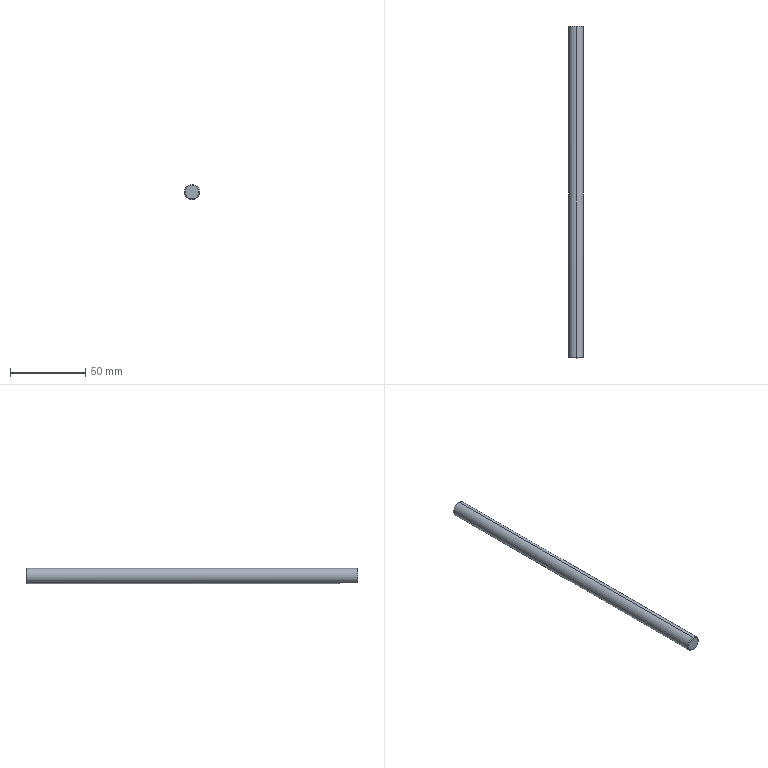Part | SolidWorks | features Chamfer 1, Extrusion 1, ICE 1 | 1 solid | 10 faces | box 10 x 220 x 10 mm | volume 17254 mm3 | cone 4 | plane 4 | cylinder 2 | commonest cylinder face diameters 10 x2
STEP:
#1=CARTESIAN_POINT('',(0.,220.,4.5));
#2=VERTEX_POINT('',#1);
#3=CARTESIAN_POINT('',(0.,220.,-4.5));
#4=VERTEX_POINT('',#3);
#5=CARTESIAN_POINT('',(0.,220.,0.));
#6=DIRECTION('',(0.,1.,0.));
#7=DIRECTION('',(0.,0.,1.));
#8=AXIS2_PLACEMENT_3D('',#5,#6,#7);
#9=CIRCLE('',#8,4.5);
#10=EDGE_CURVE('',#2,#4,#9,.T.);
#11=ORIENTED_EDGE('',*,*,#10,.F.);
#12=CARTESIAN_POINT('',(0.,219.5,5.));
#13=VERTEX_POINT('',#12);
#14=CARTESIAN_POINT('',(0.,220.,4.5));
#15=DIRECTION('',(0.,-0.7071,0.7071));
#16=VECTOR('',#15,1000.);
#17=LINE('',#14,#16);
#18=EDGE_CURVE('',#2,#13,#17,.T.);
#19=ORIENTED_EDGE('',*,*,#18,.T.);
#20=CARTESIAN_POINT('',(0.,219.5,-5.));
#21=VERTEX_POINT('',#20);
#22=CARTESIAN_POINT('',(0.,219.5,0.));
#23=DIRECTION('',(0.,-1.,0.));
#24=DIRECTION('',(0.,0.,1.));
#25=AXIS2_PLACEMENT_3D('',#22,#23,#24);
#26=CIRCLE('',#25,5.);
#27=EDGE_CURVE('',#21,#13,#26,.T.);
#28=ORIENTED_EDGE('',*,*,#27,.F.);
#29=CARTESIAN_POINT('',(0.,220.,-4.5));
#30=DIRECTION('',(0.,-0.7071,-0.7071));
#31=VECTOR('',#30,1000.);
#32=LINE('',#29,#31);
#33=EDGE_CURVE('',#4,#21,#32,.T.);
#34=ORIENTED_EDGE('',*,*,#33,.F.);
#35=EDGE_LOOP('',(#11,#19,#28,#34));
#36=FACE_OUTER_BOUND('',#35,.T.);
#37=CARTESIAN_POINT('',(0.,220.,0.));
#38=DIRECTION('',(0.,-1.,0.));
#39=DIRECTION('',(0.,0.,-1.));
#40=AXIS2_PLACEMENT_3D('',#37,#38,#39);
#41=CONICAL_SURFACE('',#40,4.5,0.7854);
#42=ADVANCED_FACE('',(#36),#41,.T.);
#43=CARTESIAN_POINT('',(0.,0.,4.5));
#44=VERTEX_POINT('',#43);
#45=CARTESIAN_POINT('',(0.,0.,-4.5));
#46=VERTEX_POINT('',#45);
#47=CARTESIAN_POINT('',(0.,0.,0.));
#48=DIRECTION('',(0.,-1.,0.));
#49=DIRECTION('',(0.,0.,1.));
#50=AXIS2_PLACEMENT_3D('',#47,#48,#49);
#51=CIRCLE('',#50,4.5);
#52=EDGE_CURVE('',#44,#46,#51,.T.);
#53=ORIENTED_EDGE('',*,*,#52,.F.);
#54=CARTESIAN_POINT('',(0.,0.5,5.));
#55=VERTEX_POINT('',#54);
#56=CARTESIAN_POINT('',(0.,0.5,5.));
#57=DIRECTION('',(0.,0.7071,0.7071));
#58=VECTOR('',#57,1000.);
#59=LINE('',#56,#58);
#60=EDGE_CURVE('',#44,#55,#59,.T.);
#61=ORIENTED_EDGE('',*,*,#60,.T.);
#62=CARTESIAN_POINT('',(-2.179,0.5,-4.5));
#63=VERTEX_POINT('',#62);
#64=CARTESIAN_POINT('',(0.,0.5,0.));
#65=DIRECTION('',(0.,1.,0.));
#66=DIRECTION('',(0.,0.,1.));
#67=AXIS2_PLACEMENT_3D('',#64,#65,#66);
#68=CIRCLE('',#67,5.);
#69=EDGE_CURVE('',#63,#55,#68,.T.);
#70=ORIENTED_EDGE('',*,*,#69,.F.);
#71=CARTESIAN_POINT('',(-2.179,0.5,-4.5));
#72=CARTESIAN_POINT('',(-1.837,0.3506,-4.5));
#73=CARTESIAN_POINT('',(-1.477,0.2231,-4.5));
#74=CARTESIAN_POINT('',(-0.7491,0.04821,-4.5));
#75=CARTESIAN_POINT('',(-0.3785,0.,-4.5));
#76=CARTESIAN_POINT('',(0.,0.,-4.5));
#77=B_SPLINE_CURVE_WITH_KNOTS('',3,(#71,#72,#73,#74,#75,#76),.UNSPECIFIED.,.F.,.F.,(4,2,4),(0.002939,0.004056,0.005172),.UNSPECIFIED.);
#78=EDGE_CURVE('',#63,#46,#77,.T.);
#79=ORIENTED_EDGE('',*,*,#78,.T.);
#80=EDGE_LOOP('',(#53,#61,#70,#79));
#81=FACE_OUTER_BOUND('',#80,.T.);
#82=CARTESIAN_POINT('',(0.,0.5,0.));
#83=DIRECTION('',(0.,1.,0.));
#84=DIRECTION('',(0.,0.,1.));
#85=AXIS2_PLACEMENT_3D('',#82,#83,#84);
#86=CONICAL_SURFACE('',#85,5.,0.7854);
#87=ADVANCED_FACE('',(#81),#86,.T.);
#88=ORIENTED_EDGE('',*,*,#27,.T.);
#89=CARTESIAN_POINT('',(0.,220.,5.));
#90=DIRECTION('',(0.,-1.,0.));
#91=VECTOR('',#90,1000.);
#92=LINE('',#89,#91);
#93=EDGE_CURVE('',#13,#55,#92,.T.);
#94=ORIENTED_EDGE('',*,*,#93,.T.);
#95=CARTESIAN_POINT('',(2.179,0.5,-4.5));
#96=VERTEX_POINT('',#95);
#97=CARTESIAN_POINT('',(0.,0.5,0.));
#98=DIRECTION('',(0.,1.,0.));
#99=DIRECTION('',(0.,0.,1.));
#100=AXIS2_PLACEMENT_3D('',#97,#98,#99);
#101=CIRCLE('',#100,5.);
#102=EDGE_CURVE('',#55,#96,#101,.T.);
#103=ORIENTED_EDGE('',*,*,#102,.T.);
#104=CARTESIAN_POINT('',(2.179,12.,-4.5));
#105=VERTEX_POINT('',#104);
#106=CARTESIAN_POINT('',(2.179,12.,-4.5));
#107=DIRECTION('',(0.,-1.,0.));
#108=VECTOR('',#107,1000.);
#109=LINE('',#106,#108);
#110=EDGE_CURVE('',#105,#96,#109,.T.);
#111=ORIENTED_EDGE('',*,*,#110,.F.);
#112=CARTESIAN_POINT('',(0.,12.,-5.));
#113=VERTEX_POINT('',#112);
#114=CARTESIAN_POINT('',(0.,12.,0.));
#115=DIRECTION('',(0.,1.,0.));
#116=DIRECTION('',(0.,0.,1.));
#117=AXIS2_PLACEMENT_3D('',#114,#115,#116);
#118=CIRCLE('',#117,5.);
#119=EDGE_CURVE('',#105,#113,#118,.T.);
#120=ORIENTED_EDGE('',*,*,#119,.T.);
#121=CARTESIAN_POINT('',(0.,220.,-5.));
#122=DIRECTION('',(0.,-1.,0.));
#123=VECTOR('',#122,1000.);
#124=LINE('',#121,#123);
#125=EDGE_CURVE('',#21,#113,#124,.T.);
#126=ORIENTED_EDGE('',*,*,#125,.F.);
#127=EDGE_LOOP('',(#88,#94,#103,#111,#120,#126));
#128=FACE_OUTER_BOUND('',#127,.T.);
#129=CARTESIAN_POINT('',(0.,220.,0.));
#130=DIRECTION('',(0.,-1.,0.));
#131=DIRECTION('',(0.,0.,-1.));
#132=AXIS2_PLACEMENT_3D('',#129,#130,#131);
#133=CYLINDRICAL_SURFACE('',#132,5.);
#134=ADVANCED_FACE('',(#128),#133,.T.);
#135=ORIENTED_EDGE('',*,*,#93,.F.);
#136=CARTESIAN_POINT('',(0.,219.5,0.));
#137=DIRECTION('',(0.,-1.,0.));
#138=DIRECTION('',(0.,0.,1.));
#139=AXIS2_PLACEMENT_3D('',#136,#137,#138);
#140=CIRCLE('',#139,5.);
#141=EDGE_CURVE('',#13,#21,#140,.T.);
#142=ORIENTED_EDGE('',*,*,#141,.T.);
#143=ORIENTED_EDGE('',*,*,#125,.T.);
#144=CARTESIAN_POINT('',(-2.179,12.,-4.5));
#145=VERTEX_POINT('',#144);
#146=CARTESIAN_POINT('',(0.,12.,0.));
#147=DIRECTION('',(0.,1.,0.));
#148=DIRECTION('',(0.,0.,1.));
#149=AXIS2_PLACEMENT_3D('',#146,#147,#148);
#150=CIRCLE('',#149,5.);
#151=EDGE_CURVE('',#113,#145,#150,.T.);
#152=ORIENTED_EDGE('',*,*,#151,.T.);
#153=CARTESIAN_POINT('',(-2.179,12.,-4.5));
#154=DIRECTION('',(0.,-1.,0.));
#155=VECTOR('',#154,1000.);
#156=LINE('',#153,#155);
#157=EDGE_CURVE('',#145,#63,#156,.T.);
#158=ORIENTED_EDGE('',*,*,#157,.T.);
#159=ORIENTED_EDGE('',*,*,#69,.T.);
#160=EDGE_LOOP('',(#135,#142,#143,#152,#158,#159));
#161=FACE_OUTER_BOUND('',#160,.T.);
#162=CARTESIAN_POINT('',(0.,220.,0.));
#163=DIRECTION('',(0.,-1.,0.));
#164=DIRECTION('',(0.,0.,-1.));
#165=AXIS2_PLACEMENT_3D('',#162,#163,#164);
#166=CYLINDRICAL_SURFACE('',#165,5.);
#167=ADVANCED_FACE('',(#161),#166,.T.);
#168=ORIENTED_EDGE('',*,*,#60,.F.);
#169=CARTESIAN_POINT('',(0.,0.,0.));
#170=DIRECTION('',(0.,-1.,0.));
#171=DIRECTION('',(0.,0.,1.));
#172=AXIS2_PLACEMENT_3D('',#169,#170,#171);
#173=CIRCLE('',#172,4.5);
#174=EDGE_CURVE('',#46,#44,#173,.T.);
#175=ORIENTED_EDGE('',*,*,#174,.F.);
#176=CARTESIAN_POINT('',(0.,0.,-4.5));
#177=CARTESIAN_POINT('',(0.3779,0.,-4.5));
#178=CARTESIAN_POINT('',(0.7513,0.04863,-4.5));
#179=CARTESIAN_POINT('',(1.478,0.2234,-4.5));
#180=CARTESIAN_POINT('',(1.836,0.3505,-4.5));
#181=CARTESIAN_POINT('',(2.179,0.5,-4.5));
#182=B_SPLINE_CURVE_WITH_KNOTS('',3,(#176,#177,#178,#179,#180,#181),.UNSPECIFIED.,.F.,.F.,(4,2,4),(0.005172,0.006287,0.007401),.UNSPECIFIED.);
#183=EDGE_CURVE('',#46,#96,#182,.T.);
#184=ORIENTED_EDGE('',*,*,#183,.T.);
#185=ORIENTED_EDGE('',*,*,#102,.F.);
#186=EDGE_LOOP('',(#168,#175,#184,#185));
#187=FACE_OUTER_BOUND('',#186,.T.);
#188=CARTESIAN_POINT('',(0.,0.5,0.));
#189=DIRECTION('',(0.,1.,0.));
#190=DIRECTION('',(0.,0.,1.));
#191=AXIS2_PLACEMENT_3D('',#188,#189,#190);
#192=CONICAL_SURFACE('',#191,5.,0.7854);
#193=ADVANCED_FACE('',(#187),#192,.T.);
#194=CARTESIAN_POINT('',(0.,220.,0.));
#195=DIRECTION('',(0.,1.,0.));
#196=DIRECTION('',(0.,0.,1.));
#197=AXIS2_PLACEMENT_3D('',#194,#195,#196);
#198=CIRCLE('',#197,4.5);
#199=EDGE_CURVE('',#4,#2,#198,.T.);
#200=ORIENTED_EDGE('',*,*,#199,.T.);
#201=ORIENTED_EDGE('',*,*,#10,.T.);
#202=EDGE_LOOP('',(#200,#201));
#203=FACE_OUTER_BOUND('',#202,.T.);
#204=CARTESIAN_POINT('',(0.,220.,0.));
#205=DIRECTION('',(0.,1.,0.));
#206=DIRECTION('',(0.,0.,1.));
#207=AXIS2_PLACEMENT_3D('',#204,#205,#206);
#208=PLANE('',#207);
#209=ADVANCED_FACE('',(#203),#208,.T.);
#210=ORIENTED_EDGE('',*,*,#174,.T.);
#211=ORIENTED_EDGE('',*,*,#52,.T.);
#212=EDGE_LOOP('',(#210,#211));
#213=FACE_OUTER_BOUND('',#212,.T.);
#214=CARTESIAN_POINT('',(0.,0.,0.));
#215=DIRECTION('',(0.,1.,0.));
#216=DIRECTION('',(0.,0.,1.));
#217=AXIS2_PLACEMENT_3D('',#214,#215,#216);
#218=PLANE('',#217);
#219=ADVANCED_FACE('',(#213),#218,.F.);
#220=ORIENTED_EDGE('',*,*,#18,.F.);
#221=ORIENTED_EDGE('',*,*,#199,.F.);
#222=ORIENTED_EDGE('',*,*,#33,.T.);
#223=ORIENTED_EDGE('',*,*,#141,.F.);
#224=EDGE_LOOP('',(#220,#221,#222,#223));
#225=FACE_OUTER_BOUND('',#224,.T.);
#226=CARTESIAN_POINT('',(0.,220.,0.));
#227=DIRECTION('',(0.,-1.,0.));
#228=DIRECTION('',(0.,0.,-1.));
#229=AXIS2_PLACEMENT_3D('',#226,#227,#228);
#230=CONICAL_SURFACE('',#229,4.5,0.7854);
#231=ADVANCED_FACE('',(#225),#230,.T.);
#232=ORIENTED_EDGE('',*,*,#157,.F.);
#233=CARTESIAN_POINT('',(-2.179,12.,-4.5));
#234=DIRECTION('',(1.,0.,0.));
#235=VECTOR('',#234,1000.);
#236=LINE('',#233,#235);
#237=EDGE_CURVE('',#145,#105,#236,.T.);
#238=ORIENTED_EDGE('',*,*,#237,.T.);
#239=ORIENTED_EDGE('',*,*,#110,.T.);
#240=ORIENTED_EDGE('',*,*,#183,.F.);
#241=ORIENTED_EDGE('',*,*,#78,.F.);
#242=EDGE_LOOP('',(#232,#238,#239,#240,#241));
#243=FACE_OUTER_BOUND('',#242,.T.);
#244=CARTESIAN_POINT('',(-2.179,12.,-4.5));
#245=DIRECTION('',(0.,0.,-1.));
#246=DIRECTION('',(-1.,0.,0.));
#247=AXIS2_PLACEMENT_3D('',#244,#245,#246);
#248=PLANE('',#247);
#249=ADVANCED_FACE('',(#243),#248,.T.);
#250=ORIENTED_EDGE('',*,*,#119,.F.);
#251=ORIENTED_EDGE('',*,*,#237,.F.);
#252=ORIENTED_EDGE('',*,*,#151,.F.);
#253=EDGE_LOOP('',(#250,#251,#252));
#254=FACE_OUTER_BOUND('',#253,.T.);
#255=CARTESIAN_POINT('',(0.,12.,0.));
#256=DIRECTION('',(0.,1.,0.));
#257=DIRECTION('',(0.,0.,1.));
#258=AXIS2_PLACEMENT_3D('',#255,#256,#257);
#259=PLANE('',#258);
#260=ADVANCED_FACE('',(#254),#259,.F.);
#261=CLOSED_SHELL('',(#42,#87,#134,#167,#193,#209,#219,#231,#249,#260));
#262=MANIFOLD_SOLID_BREP('',#261);
#263=CARTESIAN_POINT('',(0.,0.,0.));
#264=DIRECTION('',(0.,0.,1.));
#265=DIRECTION('',(1.,0.,0.));
#266=AXIS2_PLACEMENT_3D('',#263,#264,#265);
#267=(LENGTH_UNIT()NAMED_UNIT(*)SI_UNIT(.MILLI.,.METRE.));
#268=UNCERTAINTY_MEASURE_WITH_UNIT(LENGTH_MEASURE(0.00001),#267,'','');
#269=(NAMED_UNIT(*)PLANE_ANGLE_UNIT()SI_UNIT($,.RADIAN.));
#270=(NAMED_UNIT(*)SI_UNIT($,.STERADIAN.)SOLID_ANGLE_UNIT());
#271=(GEOMETRIC_REPRESENTATION_CONTEXT(3)GLOBAL_UNCERTAINTY_ASSIGNED_CONTEXT((#268))GLOBAL_UNIT_ASSIGNED_CONTEXT((#267,#269,#270))REPRESENTATION_CONTEXT('',''));
#272=ADVANCED_BREP_SHAPE_REPRESENTATION('',(#262,#266),#271);